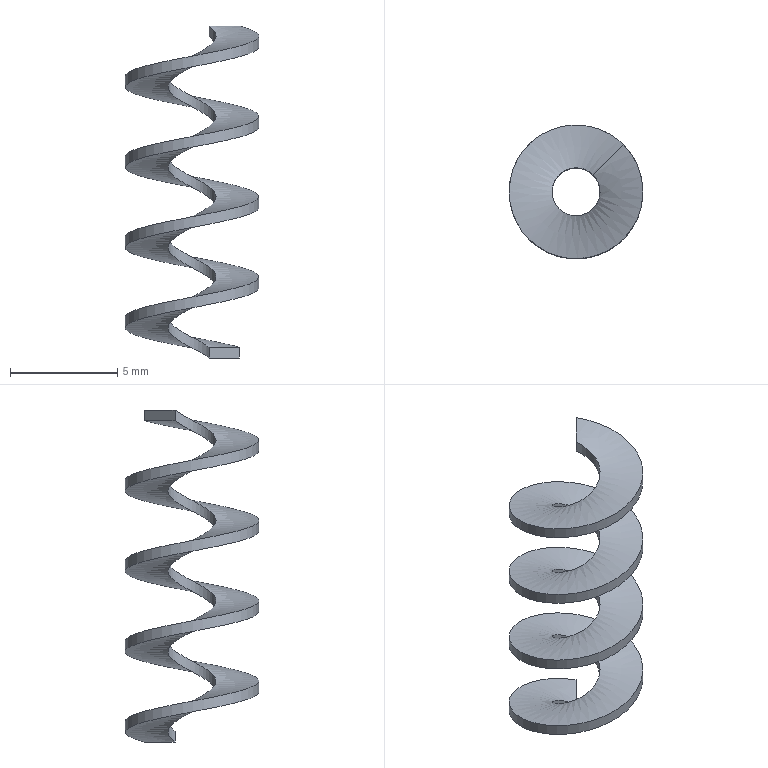Part | SolidWorks | features Helix 1, Sweep 1 | 1 solid | 6 faces | box 6.243 x 6.243 x 15.5 mm | volume 53.36 mm3 | spline 4 | plane 2